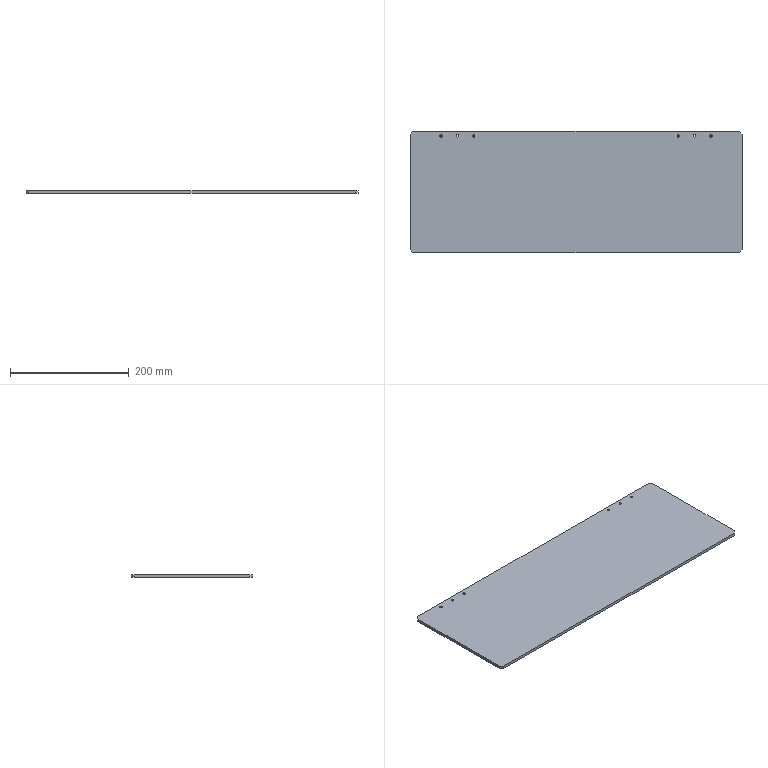Part | SolidWorks | features Extrusion 1 | 1 solid | 22 faces | box 560 x 205 x 5 mm | volume 573373 mm3 | cylinder 12 | plane 10 | commonest cylinder face diameters 4 x12
STEP:
#1=CARTESIAN_POINT('',(505.5,-8.,5.));
#2=VERTEX_POINT('',#1);
#3=CARTESIAN_POINT('',(509.5,-8.,5.));
#4=VERTEX_POINT('',#3);
#5=CARTESIAN_POINT('',(507.5,-8.,5.));
#6=DIRECTION('',(0.,0.,1.));
#7=DIRECTION('',(-1.,0.,0.));
#8=AXIS2_PLACEMENT_3D('',#5,#6,#7);
#9=CIRCLE('',#8,2.);
#10=EDGE_CURVE('',#2,#4,#9,.T.);
#11=ORIENTED_EDGE('',*,*,#10,.T.);
#12=CARTESIAN_POINT('',(509.5,-8.,0.));
#13=VERTEX_POINT('',#12);
#14=CARTESIAN_POINT('',(509.5,-8.,5.));
#15=DIRECTION('',(0.,0.,-1.));
#16=VECTOR('',#15,1000.);
#17=LINE('',#14,#16);
#18=EDGE_CURVE('',#4,#13,#17,.T.);
#19=ORIENTED_EDGE('',*,*,#18,.T.);
#20=CARTESIAN_POINT('',(505.5,-8.,0.));
#21=VERTEX_POINT('',#20);
#22=CARTESIAN_POINT('',(507.5,-8.,0.));
#23=DIRECTION('',(0.,0.,1.));
#24=DIRECTION('',(-1.,0.,0.));
#25=AXIS2_PLACEMENT_3D('',#22,#23,#24);
#26=CIRCLE('',#25,2.);
#27=EDGE_CURVE('',#21,#13,#26,.T.);
#28=ORIENTED_EDGE('',*,*,#27,.F.);
#29=CARTESIAN_POINT('',(505.5,-8.,5.));
#30=DIRECTION('',(0.,0.,-1.));
#31=VECTOR('',#30,1000.);
#32=LINE('',#29,#31);
#33=EDGE_CURVE('',#2,#21,#32,.T.);
#34=ORIENTED_EDGE('',*,*,#33,.F.);
#35=EDGE_LOOP('',(#11,#19,#28,#34));
#36=FACE_OUTER_BOUND('',#35,.T.);
#37=CARTESIAN_POINT('',(507.5,-8.,5.));
#38=DIRECTION('',(0.,0.,-1.));
#39=DIRECTION('',(-1.,0.,0.));
#40=AXIS2_PLACEMENT_3D('',#37,#38,#39);
#41=CYLINDRICAL_SURFACE('',#40,2.);
#42=ADVANCED_FACE('',(#36),#41,.F.);
#43=CARTESIAN_POINT('',(478.,-8.,5.));
#44=VERTEX_POINT('',#43);
#45=CARTESIAN_POINT('',(482.,-8.,5.));
#46=VERTEX_POINT('',#45);
#47=CARTESIAN_POINT('',(480.,-8.,5.));
#48=DIRECTION('',(0.,0.,1.));
#49=DIRECTION('',(-1.,0.,0.));
#50=AXIS2_PLACEMENT_3D('',#47,#48,#49);
#51=CIRCLE('',#50,2.);
#52=EDGE_CURVE('',#44,#46,#51,.T.);
#53=ORIENTED_EDGE('',*,*,#52,.T.);
#54=CARTESIAN_POINT('',(482.,-8.,0.));
#55=VERTEX_POINT('',#54);
#56=CARTESIAN_POINT('',(482.,-8.,5.));
#57=DIRECTION('',(0.,0.,-1.));
#58=VECTOR('',#57,1000.);
#59=LINE('',#56,#58);
#60=EDGE_CURVE('',#46,#55,#59,.T.);
#61=ORIENTED_EDGE('',*,*,#60,.T.);
#62=CARTESIAN_POINT('',(478.,-8.,0.));
#63=VERTEX_POINT('',#62);
#64=CARTESIAN_POINT('',(480.,-8.,0.));
#65=DIRECTION('',(0.,0.,1.));
#66=DIRECTION('',(-1.,0.,0.));
#67=AXIS2_PLACEMENT_3D('',#64,#65,#66);
#68=CIRCLE('',#67,2.);
#69=EDGE_CURVE('',#63,#55,#68,.T.);
#70=ORIENTED_EDGE('',*,*,#69,.F.);
#71=CARTESIAN_POINT('',(478.,-8.,5.));
#72=DIRECTION('',(0.,0.,-1.));
#73=VECTOR('',#72,1000.);
#74=LINE('',#71,#73);
#75=EDGE_CURVE('',#44,#63,#74,.T.);
#76=ORIENTED_EDGE('',*,*,#75,.F.);
#77=EDGE_LOOP('',(#53,#61,#70,#76));
#78=FACE_OUTER_BOUND('',#77,.T.);
#79=CARTESIAN_POINT('',(480.,-8.,5.));
#80=DIRECTION('',(0.,0.,-1.));
#81=DIRECTION('',(-1.,0.,0.));
#82=AXIS2_PLACEMENT_3D('',#79,#80,#81);
#83=CYLINDRICAL_SURFACE('',#82,2.);
#84=ADVANCED_FACE('',(#78),#83,.F.);
#85=CARTESIAN_POINT('',(450.5,-8.,5.));
#86=VERTEX_POINT('',#85);
#87=CARTESIAN_POINT('',(454.5,-8.,5.));
#88=VERTEX_POINT('',#87);
#89=CARTESIAN_POINT('',(452.5,-8.,5.));
#90=DIRECTION('',(0.,0.,1.));
#91=DIRECTION('',(-1.,0.,0.));
#92=AXIS2_PLACEMENT_3D('',#89,#90,#91);
#93=CIRCLE('',#92,2.);
#94=EDGE_CURVE('',#86,#88,#93,.T.);
#95=ORIENTED_EDGE('',*,*,#94,.T.);
#96=CARTESIAN_POINT('',(454.5,-8.,0.));
#97=VERTEX_POINT('',#96);
#98=CARTESIAN_POINT('',(454.5,-8.,5.));
#99=DIRECTION('',(0.,0.,-1.));
#100=VECTOR('',#99,1000.);
#101=LINE('',#98,#100);
#102=EDGE_CURVE('',#88,#97,#101,.T.);
#103=ORIENTED_EDGE('',*,*,#102,.T.);
#104=CARTESIAN_POINT('',(450.5,-8.,0.));
#105=VERTEX_POINT('',#104);
#106=CARTESIAN_POINT('',(452.5,-8.,0.));
#107=DIRECTION('',(0.,0.,1.));
#108=DIRECTION('',(-1.,0.,0.));
#109=AXIS2_PLACEMENT_3D('',#106,#107,#108);
#110=CIRCLE('',#109,2.);
#111=EDGE_CURVE('',#105,#97,#110,.T.);
#112=ORIENTED_EDGE('',*,*,#111,.F.);
#113=CARTESIAN_POINT('',(450.5,-8.,5.));
#114=DIRECTION('',(0.,0.,-1.));
#115=VECTOR('',#114,1000.);
#116=LINE('',#113,#115);
#117=EDGE_CURVE('',#86,#105,#116,.T.);
#118=ORIENTED_EDGE('',*,*,#117,.F.);
#119=EDGE_LOOP('',(#95,#103,#112,#118));
#120=FACE_OUTER_BOUND('',#119,.T.);
#121=CARTESIAN_POINT('',(452.5,-8.,5.));
#122=DIRECTION('',(0.,0.,-1.));
#123=DIRECTION('',(-1.,0.,0.));
#124=AXIS2_PLACEMENT_3D('',#121,#122,#123);
#125=CYLINDRICAL_SURFACE('',#124,2.);
#126=ADVANCED_FACE('',(#120),#125,.F.);
#127=CARTESIAN_POINT('',(105.5,-8.,5.));
#128=VERTEX_POINT('',#127);
#129=CARTESIAN_POINT('',(109.5,-8.,5.));
#130=VERTEX_POINT('',#129);
#131=CARTESIAN_POINT('',(107.5,-8.,5.));
#132=DIRECTION('',(0.,0.,1.));
#133=DIRECTION('',(1.,0.,0.));
#134=AXIS2_PLACEMENT_3D('',#131,#132,#133);
#135=CIRCLE('',#134,2.);
#136=EDGE_CURVE('',#128,#130,#135,.T.);
#137=ORIENTED_EDGE('',*,*,#136,.T.);
#138=CARTESIAN_POINT('',(109.5,-8.,0.));
#139=VERTEX_POINT('',#138);
#140=CARTESIAN_POINT('',(109.5,-8.,5.));
#141=DIRECTION('',(0.,0.,-1.));
#142=VECTOR('',#141,1000.);
#143=LINE('',#140,#142);
#144=EDGE_CURVE('',#130,#139,#143,.T.);
#145=ORIENTED_EDGE('',*,*,#144,.T.);
#146=CARTESIAN_POINT('',(105.5,-8.,0.));
#147=VERTEX_POINT('',#146);
#148=CARTESIAN_POINT('',(107.5,-8.,0.));
#149=DIRECTION('',(0.,0.,1.));
#150=DIRECTION('',(1.,0.,0.));
#151=AXIS2_PLACEMENT_3D('',#148,#149,#150);
#152=CIRCLE('',#151,2.);
#153=EDGE_CURVE('',#147,#139,#152,.T.);
#154=ORIENTED_EDGE('',*,*,#153,.F.);
#155=CARTESIAN_POINT('',(105.5,-8.,5.));
#156=DIRECTION('',(0.,0.,-1.));
#157=VECTOR('',#156,1000.);
#158=LINE('',#155,#157);
#159=EDGE_CURVE('',#128,#147,#158,.T.);
#160=ORIENTED_EDGE('',*,*,#159,.F.);
#161=EDGE_LOOP('',(#137,#145,#154,#160));
#162=FACE_OUTER_BOUND('',#161,.T.);
#163=CARTESIAN_POINT('',(107.5,-8.,5.));
#164=DIRECTION('',(0.,0.,-1.));
#165=DIRECTION('',(-1.,0.,0.));
#166=AXIS2_PLACEMENT_3D('',#163,#164,#165);
#167=CYLINDRICAL_SURFACE('',#166,2.);
#168=ADVANCED_FACE('',(#162),#167,.F.);
#169=CARTESIAN_POINT('',(78.,-8.,5.));
#170=VERTEX_POINT('',#169);
#171=CARTESIAN_POINT('',(82.,-8.,5.));
#172=VERTEX_POINT('',#171);
#173=CARTESIAN_POINT('',(80.,-8.,5.));
#174=DIRECTION('',(0.,0.,1.));
#175=DIRECTION('',(1.,0.,0.));
#176=AXIS2_PLACEMENT_3D('',#173,#174,#175);
#177=CIRCLE('',#176,2.);
#178=EDGE_CURVE('',#170,#172,#177,.T.);
#179=ORIENTED_EDGE('',*,*,#178,.T.);
#180=CARTESIAN_POINT('',(82.,-8.,0.));
#181=VERTEX_POINT('',#180);
#182=CARTESIAN_POINT('',(82.,-8.,5.));
#183=DIRECTION('',(0.,0.,-1.));
#184=VECTOR('',#183,1000.);
#185=LINE('',#182,#184);
#186=EDGE_CURVE('',#172,#181,#185,.T.);
#187=ORIENTED_EDGE('',*,*,#186,.T.);
#188=CARTESIAN_POINT('',(78.,-8.,0.));
#189=VERTEX_POINT('',#188);
#190=CARTESIAN_POINT('',(80.,-8.,0.));
#191=DIRECTION('',(0.,0.,1.));
#192=DIRECTION('',(1.,0.,0.));
#193=AXIS2_PLACEMENT_3D('',#190,#191,#192);
#194=CIRCLE('',#193,2.);
#195=EDGE_CURVE('',#189,#181,#194,.T.);
#196=ORIENTED_EDGE('',*,*,#195,.F.);
#197=CARTESIAN_POINT('',(78.,-8.,5.));
#198=DIRECTION('',(0.,0.,-1.));
#199=VECTOR('',#198,1000.);
#200=LINE('',#197,#199);
#201=EDGE_CURVE('',#170,#189,#200,.T.);
#202=ORIENTED_EDGE('',*,*,#201,.F.);
#203=EDGE_LOOP('',(#179,#187,#196,#202));
#204=FACE_OUTER_BOUND('',#203,.T.);
#205=CARTESIAN_POINT('',(80.,-8.,5.));
#206=DIRECTION('',(0.,0.,-1.));
#207=DIRECTION('',(-1.,0.,0.));
#208=AXIS2_PLACEMENT_3D('',#205,#206,#207);
#209=CYLINDRICAL_SURFACE('',#208,2.);
#210=ADVANCED_FACE('',(#204),#209,.F.);
#211=CARTESIAN_POINT('',(50.5,-8.,5.));
#212=VERTEX_POINT('',#211);
#213=CARTESIAN_POINT('',(54.5,-8.,5.));
#214=VERTEX_POINT('',#213);
#215=CARTESIAN_POINT('',(52.5,-8.,5.));
#216=DIRECTION('',(0.,0.,1.));
#217=DIRECTION('',(1.,0.,0.));
#218=AXIS2_PLACEMENT_3D('',#215,#216,#217);
#219=CIRCLE('',#218,2.);
#220=EDGE_CURVE('',#212,#214,#219,.T.);
#221=ORIENTED_EDGE('',*,*,#220,.T.);
#222=CARTESIAN_POINT('',(54.5,-8.,0.));
#223=VERTEX_POINT('',#222);
#224=CARTESIAN_POINT('',(54.5,-8.,5.));
#225=DIRECTION('',(0.,0.,-1.));
#226=VECTOR('',#225,1000.);
#227=LINE('',#224,#226);
#228=EDGE_CURVE('',#214,#223,#227,.T.);
#229=ORIENTED_EDGE('',*,*,#228,.T.);
#230=CARTESIAN_POINT('',(50.5,-8.,0.));
#231=VERTEX_POINT('',#230);
#232=CARTESIAN_POINT('',(52.5,-8.,0.));
#233=DIRECTION('',(0.,0.,1.));
#234=DIRECTION('',(1.,0.,0.));
#235=AXIS2_PLACEMENT_3D('',#232,#233,#234);
#236=CIRCLE('',#235,2.);
#237=EDGE_CURVE('',#231,#223,#236,.T.);
#238=ORIENTED_EDGE('',*,*,#237,.F.);
#239=CARTESIAN_POINT('',(50.5,-8.,5.));
#240=DIRECTION('',(0.,0.,-1.));
#241=VECTOR('',#240,1000.);
#242=LINE('',#239,#241);
#243=EDGE_CURVE('',#212,#231,#242,.T.);
#244=ORIENTED_EDGE('',*,*,#243,.F.);
#245=EDGE_LOOP('',(#221,#229,#238,#244));
#246=FACE_OUTER_BOUND('',#245,.T.);
#247=CARTESIAN_POINT('',(52.5,-8.,5.));
#248=DIRECTION('',(0.,0.,-1.));
#249=DIRECTION('',(-1.,0.,0.));
#250=AXIS2_PLACEMENT_3D('',#247,#248,#249);
#251=CYLINDRICAL_SURFACE('',#250,2.);
#252=ADVANCED_FACE('',(#246),#251,.F.);
#253=CARTESIAN_POINT('',(555.,0.,5.));
#254=VERTEX_POINT('',#253);
#255=CARTESIAN_POINT('',(5.,0.,5.));
#256=VERTEX_POINT('',#255);
#257=CARTESIAN_POINT('',(5.,0.,5.));
#258=DIRECTION('',(-1.,0.,0.));
#259=VECTOR('',#258,1000.);
#260=LINE('',#257,#259);
#261=EDGE_CURVE('',#254,#256,#260,.T.);
#262=ORIENTED_EDGE('',*,*,#261,.T.);
#263=CARTESIAN_POINT('',(0.,-5.,5.));
#264=VERTEX_POINT('',#263);
#265=CARTESIAN_POINT('',(0.,-5.,5.));
#266=DIRECTION('',(-0.7071,-0.7071,0.));
#267=VECTOR('',#266,1000.);
#268=LINE('',#265,#267);
#269=EDGE_CURVE('',#256,#264,#268,.T.);
#270=ORIENTED_EDGE('',*,*,#269,.T.);
#271=CARTESIAN_POINT('',(0.,-200.,5.));
#272=VERTEX_POINT('',#271);
#273=CARTESIAN_POINT('',(0.,-5.,5.));
#274=DIRECTION('',(0.,-1.,0.));
#275=VECTOR('',#274,1000.);
#276=LINE('',#273,#275);
#277=EDGE_CURVE('',#264,#272,#276,.T.);
#278=ORIENTED_EDGE('',*,*,#277,.T.);
#279=CARTESIAN_POINT('',(5.,-205.,5.));
#280=VERTEX_POINT('',#279);
#281=CARTESIAN_POINT('',(0.,-200.,5.));
#282=DIRECTION('',(0.7071,-0.7071,0.));
#283=VECTOR('',#282,1000.);
#284=LINE('',#281,#283);
#285=EDGE_CURVE('',#272,#280,#284,.T.);
#286=ORIENTED_EDGE('',*,*,#285,.T.);
#287=CARTESIAN_POINT('',(555.,-205.,5.));
#288=VERTEX_POINT('',#287);
#289=CARTESIAN_POINT('',(5.,-205.,5.));
#290=DIRECTION('',(1.,0.,0.));
#291=VECTOR('',#290,1000.);
#292=LINE('',#289,#291);
#293=EDGE_CURVE('',#280,#288,#292,.T.);
#294=ORIENTED_EDGE('',*,*,#293,.T.);
#295=CARTESIAN_POINT('',(560.,-200.,5.));
#296=VERTEX_POINT('',#295);
#297=CARTESIAN_POINT('',(560.,-200.,5.));
#298=DIRECTION('',(0.7071,0.7071,0.));
#299=VECTOR('',#298,1000.);
#300=LINE('',#297,#299);
#301=EDGE_CURVE('',#288,#296,#300,.T.);
#302=ORIENTED_EDGE('',*,*,#301,.T.);
#303=CARTESIAN_POINT('',(560.,-5.,5.));
#304=VERTEX_POINT('',#303);
#305=CARTESIAN_POINT('',(560.,-5.,5.));
#306=DIRECTION('',(0.,1.,0.));
#307=VECTOR('',#306,1000.);
#308=LINE('',#305,#307);
#309=EDGE_CURVE('',#296,#304,#308,.T.);
#310=ORIENTED_EDGE('',*,*,#309,.T.);
#311=CARTESIAN_POINT('',(555.,0.,5.));
#312=DIRECTION('',(-0.7071,0.7071,0.));
#313=VECTOR('',#312,1000.);
#314=LINE('',#311,#313);
#315=EDGE_CURVE('',#304,#254,#314,.T.);
#316=ORIENTED_EDGE('',*,*,#315,.T.);
#317=EDGE_LOOP('',(#262,#270,#278,#286,#294,#302,#310,#316));
#318=FACE_OUTER_BOUND('',#317,.T.);
#319=ORIENTED_EDGE('',*,*,#220,.F.);
#320=CARTESIAN_POINT('',(52.5,-8.,5.));
#321=DIRECTION('',(0.,0.,1.));
#322=DIRECTION('',(1.,0.,0.));
#323=AXIS2_PLACEMENT_3D('',#320,#321,#322);
#324=CIRCLE('',#323,2.);
#325=EDGE_CURVE('',#214,#212,#324,.T.);
#326=ORIENTED_EDGE('',*,*,#325,.F.);
#327=EDGE_LOOP('',(#319,#326));
#328=FACE_BOUND('',#327,.T.);
#329=ORIENTED_EDGE('',*,*,#178,.F.);
#330=CARTESIAN_POINT('',(80.,-8.,5.));
#331=DIRECTION('',(0.,0.,1.));
#332=DIRECTION('',(1.,0.,0.));
#333=AXIS2_PLACEMENT_3D('',#330,#331,#332);
#334=CIRCLE('',#333,2.);
#335=EDGE_CURVE('',#172,#170,#334,.T.);
#336=ORIENTED_EDGE('',*,*,#335,.F.);
#337=EDGE_LOOP('',(#329,#336));
#338=FACE_BOUND('',#337,.T.);
#339=ORIENTED_EDGE('',*,*,#136,.F.);
#340=CARTESIAN_POINT('',(107.5,-8.,5.));
#341=DIRECTION('',(0.,0.,1.));
#342=DIRECTION('',(1.,0.,0.));
#343=AXIS2_PLACEMENT_3D('',#340,#341,#342);
#344=CIRCLE('',#343,2.);
#345=EDGE_CURVE('',#130,#128,#344,.T.);
#346=ORIENTED_EDGE('',*,*,#345,.F.);
#347=EDGE_LOOP('',(#339,#346));
#348=FACE_BOUND('',#347,.T.);
#349=ORIENTED_EDGE('',*,*,#94,.F.);
#350=CARTESIAN_POINT('',(452.5,-8.,5.));
#351=DIRECTION('',(0.,0.,1.));
#352=DIRECTION('',(-1.,0.,0.));
#353=AXIS2_PLACEMENT_3D('',#350,#351,#352);
#354=CIRCLE('',#353,2.);
#355=EDGE_CURVE('',#88,#86,#354,.T.);
#356=ORIENTED_EDGE('',*,*,#355,.F.);
#357=EDGE_LOOP('',(#349,#356));
#358=FACE_BOUND('',#357,.T.);
#359=ORIENTED_EDGE('',*,*,#52,.F.);
#360=CARTESIAN_POINT('',(480.,-8.,5.));
#361=DIRECTION('',(0.,0.,1.));
#362=DIRECTION('',(-1.,0.,0.));
#363=AXIS2_PLACEMENT_3D('',#360,#361,#362);
#364=CIRCLE('',#363,2.);
#365=EDGE_CURVE('',#46,#44,#364,.T.);
#366=ORIENTED_EDGE('',*,*,#365,.F.);
#367=EDGE_LOOP('',(#359,#366));
#368=FACE_BOUND('',#367,.T.);
#369=ORIENTED_EDGE('',*,*,#10,.F.);
#370=CARTESIAN_POINT('',(507.5,-8.,5.));
#371=DIRECTION('',(0.,0.,1.));
#372=DIRECTION('',(-1.,0.,0.));
#373=AXIS2_PLACEMENT_3D('',#370,#371,#372);
#374=CIRCLE('',#373,2.);
#375=EDGE_CURVE('',#4,#2,#374,.T.);
#376=ORIENTED_EDGE('',*,*,#375,.F.);
#377=EDGE_LOOP('',(#369,#376));
#378=FACE_BOUND('',#377,.T.);
#379=CARTESIAN_POINT('',(0.,0.,5.));
#380=DIRECTION('',(0.,0.,-1.));
#381=DIRECTION('',(-1.,0.,0.));
#382=AXIS2_PLACEMENT_3D('',#379,#380,#381);
#383=PLANE('',#382);
#384=ADVANCED_FACE('',(#318,#328,#338,#348,#358,#368,#378),#383,.F.);
#385=ORIENTED_EDGE('',*,*,#69,.T.);
#386=CARTESIAN_POINT('',(480.,-8.,0.));
#387=DIRECTION('',(0.,0.,1.));
#388=DIRECTION('',(-1.,0.,0.));
#389=AXIS2_PLACEMENT_3D('',#386,#387,#388);
#390=CIRCLE('',#389,2.);
#391=EDGE_CURVE('',#55,#63,#390,.T.);
#392=ORIENTED_EDGE('',*,*,#391,.T.);
#393=EDGE_LOOP('',(#385,#392));
#394=FACE_BOUND('',#393,.T.);
#395=ORIENTED_EDGE('',*,*,#153,.T.);
#396=CARTESIAN_POINT('',(107.5,-8.,0.));
#397=DIRECTION('',(0.,0.,1.));
#398=DIRECTION('',(1.,0.,0.));
#399=AXIS2_PLACEMENT_3D('',#396,#397,#398);
#400=CIRCLE('',#399,2.);
#401=EDGE_CURVE('',#139,#147,#400,.T.);
#402=ORIENTED_EDGE('',*,*,#401,.T.);
#403=EDGE_LOOP('',(#395,#402));
#404=FACE_BOUND('',#403,.T.);
#405=ORIENTED_EDGE('',*,*,#237,.T.);
#406=CARTESIAN_POINT('',(52.5,-8.,0.));
#407=DIRECTION('',(0.,0.,1.));
#408=DIRECTION('',(1.,0.,0.));
#409=AXIS2_PLACEMENT_3D('',#406,#407,#408);
#410=CIRCLE('',#409,2.);
#411=EDGE_CURVE('',#223,#231,#410,.T.);
#412=ORIENTED_EDGE('',*,*,#411,.T.);
#413=EDGE_LOOP('',(#405,#412));
#414=FACE_BOUND('',#413,.T.);
#415=CARTESIAN_POINT('',(555.,0.,0.));
#416=VERTEX_POINT('',#415);
#417=CARTESIAN_POINT('',(5.,0.,0.));
#418=VERTEX_POINT('',#417);
#419=CARTESIAN_POINT('',(5.,0.,0.));
#420=DIRECTION('',(-1.,0.,0.));
#421=VECTOR('',#420,1000.);
#422=LINE('',#419,#421);
#423=EDGE_CURVE('',#416,#418,#422,.T.);
#424=ORIENTED_EDGE('',*,*,#423,.F.);
#425=CARTESIAN_POINT('',(560.,-5.,0.));
#426=VERTEX_POINT('',#425);
#427=CARTESIAN_POINT('',(555.,0.,0.));
#428=DIRECTION('',(-0.7071,0.7071,0.));
#429=VECTOR('',#428,1000.);
#430=LINE('',#427,#429);
#431=EDGE_CURVE('',#426,#416,#430,.T.);
#432=ORIENTED_EDGE('',*,*,#431,.F.);
#433=CARTESIAN_POINT('',(560.,-200.,0.));
#434=VERTEX_POINT('',#433);
#435=CARTESIAN_POINT('',(560.,-5.,0.));
#436=DIRECTION('',(0.,1.,0.));
#437=VECTOR('',#436,1000.);
#438=LINE('',#435,#437);
#439=EDGE_CURVE('',#434,#426,#438,.T.);
#440=ORIENTED_EDGE('',*,*,#439,.F.);
#441=CARTESIAN_POINT('',(555.,-205.,0.));
#442=VERTEX_POINT('',#441);
#443=CARTESIAN_POINT('',(560.,-200.,0.));
#444=DIRECTION('',(0.7071,0.7071,0.));
#445=VECTOR('',#444,1000.);
#446=LINE('',#443,#445);
#447=EDGE_CURVE('',#442,#434,#446,.T.);
#448=ORIENTED_EDGE('',*,*,#447,.F.);
#449=CARTESIAN_POINT('',(5.,-205.,0.));
#450=VERTEX_POINT('',#449);
#451=CARTESIAN_POINT('',(5.,-205.,0.));
#452=DIRECTION('',(1.,0.,0.));
#453=VECTOR('',#452,1000.);
#454=LINE('',#451,#453);
#455=EDGE_CURVE('',#450,#442,#454,.T.);
#456=ORIENTED_EDGE('',*,*,#455,.F.);
#457=CARTESIAN_POINT('',(0.,-200.,0.));
#458=VERTEX_POINT('',#457);
#459=CARTESIAN_POINT('',(0.,-200.,0.));
#460=DIRECTION('',(0.7071,-0.7071,0.));
#461=VECTOR('',#460,1000.);
#462=LINE('',#459,#461);
#463=EDGE_CURVE('',#458,#450,#462,.T.);
#464=ORIENTED_EDGE('',*,*,#463,.F.);
#465=CARTESIAN_POINT('',(0.,-5.,0.));
#466=VERTEX_POINT('',#465);
#467=CARTESIAN_POINT('',(0.,-5.,0.));
#468=DIRECTION('',(0.,-1.,0.));
#469=VECTOR('',#468,1000.);
#470=LINE('',#467,#469);
#471=EDGE_CURVE('',#466,#458,#470,.T.);
#472=ORIENTED_EDGE('',*,*,#471,.F.);
#473=CARTESIAN_POINT('',(0.,-5.,0.));
#474=DIRECTION('',(-0.7071,-0.7071,0.));
#475=VECTOR('',#474,1000.);
#476=LINE('',#473,#475);
#477=EDGE_CURVE('',#418,#466,#476,.T.);
#478=ORIENTED_EDGE('',*,*,#477,.F.);
#479=EDGE_LOOP('',(#424,#432,#440,#448,#456,#464,#472,#478));
#480=FACE_OUTER_BOUND('',#479,.T.);
#481=ORIENTED_EDGE('',*,*,#195,.T.);
#482=CARTESIAN_POINT('',(80.,-8.,0.));
#483=DIRECTION('',(0.,0.,1.));
#484=DIRECTION('',(1.,0.,0.));
#485=AXIS2_PLACEMENT_3D('',#482,#483,#484);
#486=CIRCLE('',#485,2.);
#487=EDGE_CURVE('',#181,#189,#486,.T.);
#488=ORIENTED_EDGE('',*,*,#487,.T.);
#489=EDGE_LOOP('',(#481,#488));
#490=FACE_BOUND('',#489,.T.);
#491=ORIENTED_EDGE('',*,*,#111,.T.);
#492=CARTESIAN_POINT('',(452.5,-8.,0.));
#493=DIRECTION('',(0.,0.,1.));
#494=DIRECTION('',(-1.,0.,0.));
#495=AXIS2_PLACEMENT_3D('',#492,#493,#494);
#496=CIRCLE('',#495,2.);
#497=EDGE_CURVE('',#97,#105,#496,.T.);
#498=ORIENTED_EDGE('',*,*,#497,.T.);
#499=EDGE_LOOP('',(#491,#498));
#500=FACE_BOUND('',#499,.T.);
#501=ORIENTED_EDGE('',*,*,#27,.T.);
#502=CARTESIAN_POINT('',(507.5,-8.,0.));
#503=DIRECTION('',(0.,0.,1.));
#504=DIRECTION('',(-1.,0.,0.));
#505=AXIS2_PLACEMENT_3D('',#502,#503,#504);
#506=CIRCLE('',#505,2.);
#507=EDGE_CURVE('',#13,#21,#506,.T.);
#508=ORIENTED_EDGE('',*,*,#507,.T.);
#509=EDGE_LOOP('',(#501,#508));
#510=FACE_BOUND('',#509,.T.);
#511=CARTESIAN_POINT('',(0.,0.,0.));
#512=DIRECTION('',(0.,0.,-1.));
#513=DIRECTION('',(-1.,0.,0.));
#514=AXIS2_PLACEMENT_3D('',#511,#512,#513);
#515=PLANE('',#514);
#516=ADVANCED_FACE('',(#394,#404,#414,#480,#490,#500,#510),#515,.T.);
#517=ORIENTED_EDGE('',*,*,#423,.T.);
#518=CARTESIAN_POINT('',(5.,0.,5.));
#519=DIRECTION('',(0.,0.,-1.));
#520=VECTOR('',#519,1000.);
#521=LINE('',#518,#520);
#522=EDGE_CURVE('',#256,#418,#521,.T.);
#523=ORIENTED_EDGE('',*,*,#522,.F.);
#524=ORIENTED_EDGE('',*,*,#261,.F.);
#525=CARTESIAN_POINT('',(555.,0.,5.));
#526=DIRECTION('',(0.,0.,-1.));
#527=VECTOR('',#526,1000.);
#528=LINE('',#525,#527);
#529=EDGE_CURVE('',#254,#416,#528,.T.);
#530=ORIENTED_EDGE('',*,*,#529,.T.);
#531=EDGE_LOOP('',(#517,#523,#524,#530));
#532=FACE_OUTER_BOUND('',#531,.T.);
#533=CARTESIAN_POINT('',(5.,0.,5.));
#534=DIRECTION('',(0.,-1.,0.));
#535=DIRECTION('',(1.,0.,0.));
#536=AXIS2_PLACEMENT_3D('',#533,#534,#535);
#537=PLANE('',#536);
#538=ADVANCED_FACE('',(#532),#537,.F.);
#539=ORIENTED_EDGE('',*,*,#477,.T.);
#540=CARTESIAN_POINT('',(0.,-5.,5.));
#541=DIRECTION('',(0.,0.,-1.));
#542=VECTOR('',#541,1000.);
#543=LINE('',#540,#542);
#544=EDGE_CURVE('',#264,#466,#543,.T.);
#545=ORIENTED_EDGE('',*,*,#544,.F.);
#546=ORIENTED_EDGE('',*,*,#269,.F.);
#547=ORIENTED_EDGE('',*,*,#522,.T.);
#548=EDGE_LOOP('',(#539,#545,#546,#547));
#549=FACE_OUTER_BOUND('',#548,.T.);
#550=CARTESIAN_POINT('',(0.,-5.,5.));
#551=DIRECTION('',(0.7071,-0.7071,0.));
#552=DIRECTION('',(0.7071,0.7071,0.));
#553=AXIS2_PLACEMENT_3D('',#550,#551,#552);
#554=PLANE('',#553);
#555=ADVANCED_FACE('',(#549),#554,.F.);
#556=ORIENTED_EDGE('',*,*,#471,.T.);
#557=CARTESIAN_POINT('',(0.,-200.,5.));
#558=DIRECTION('',(0.,0.,-1.));
#559=VECTOR('',#558,1000.);
#560=LINE('',#557,#559);
#561=EDGE_CURVE('',#272,#458,#560,.T.);
#562=ORIENTED_EDGE('',*,*,#561,.F.);
#563=ORIENTED_EDGE('',*,*,#277,.F.);
#564=ORIENTED_EDGE('',*,*,#544,.T.);
#565=EDGE_LOOP('',(#556,#562,#563,#564));
#566=FACE_OUTER_BOUND('',#565,.T.);
#567=CARTESIAN_POINT('',(0.,-5.,5.));
#568=DIRECTION('',(1.,0.,0.));
#569=DIRECTION('',(0.,1.,0.));
#570=AXIS2_PLACEMENT_3D('',#567,#568,#569);
#571=PLANE('',#570);
#572=ADVANCED_FACE('',(#566),#571,.F.);
#573=ORIENTED_EDGE('',*,*,#463,.T.);
#574=CARTESIAN_POINT('',(5.,-205.,5.));
#575=DIRECTION('',(0.,0.,-1.));
#576=VECTOR('',#575,1000.);
#577=LINE('',#574,#576);
#578=EDGE_CURVE('',#280,#450,#577,.T.);
#579=ORIENTED_EDGE('',*,*,#578,.F.);
#580=ORIENTED_EDGE('',*,*,#285,.F.);
#581=ORIENTED_EDGE('',*,*,#561,.T.);
#582=EDGE_LOOP('',(#573,#579,#580,#581));
#583=FACE_OUTER_BOUND('',#582,.T.);
#584=CARTESIAN_POINT('',(0.,-200.,5.));
#585=DIRECTION('',(0.7071,0.7071,0.));
#586=DIRECTION('',(-0.7071,0.7071,0.));
#587=AXIS2_PLACEMENT_3D('',#584,#585,#586);
#588=PLANE('',#587);
#589=ADVANCED_FACE('',(#583),#588,.F.);
#590=ORIENTED_EDGE('',*,*,#455,.T.);
#591=CARTESIAN_POINT('',(555.,-205.,5.));
#592=DIRECTION('',(0.,0.,-1.));
#593=VECTOR('',#592,1000.);
#594=LINE('',#591,#593);
#595=EDGE_CURVE('',#288,#442,#594,.T.);
#596=ORIENTED_EDGE('',*,*,#595,.F.);
#597=ORIENTED_EDGE('',*,*,#293,.F.);
#598=ORIENTED_EDGE('',*,*,#578,.T.);
#599=EDGE_LOOP('',(#590,#596,#597,#598));
#600=FACE_OUTER_BOUND('',#599,.T.);
#601=CARTESIAN_POINT('',(5.,-205.,5.));
#602=DIRECTION('',(0.,1.,0.));
#603=DIRECTION('',(0.,0.,1.));
#604=AXIS2_PLACEMENT_3D('',#601,#602,#603);
#605=PLANE('',#604);
#606=ADVANCED_FACE('',(#600),#605,.F.);
#607=ORIENTED_EDGE('',*,*,#447,.T.);
#608=CARTESIAN_POINT('',(560.,-200.,5.));
#609=DIRECTION('',(0.,0.,-1.));
#610=VECTOR('',#609,1000.);
#611=LINE('',#608,#610);
#612=EDGE_CURVE('',#296,#434,#611,.T.);
#613=ORIENTED_EDGE('',*,*,#612,.F.);
#614=ORIENTED_EDGE('',*,*,#301,.F.);
#615=ORIENTED_EDGE('',*,*,#595,.T.);
#616=EDGE_LOOP('',(#607,#613,#614,#615));
#617=FACE_OUTER_BOUND('',#616,.T.);
#618=CARTESIAN_POINT('',(560.,-200.,5.));
#619=DIRECTION('',(-0.7071,0.7071,0.));
#620=DIRECTION('',(-0.7071,-0.7071,0.));
#621=AXIS2_PLACEMENT_3D('',#618,#619,#620);
#622=PLANE('',#621);
#623=ADVANCED_FACE('',(#617),#622,.F.);
#624=ORIENTED_EDGE('',*,*,#439,.T.);
#625=CARTESIAN_POINT('',(560.,-5.,5.));
#626=DIRECTION('',(0.,0.,-1.));
#627=VECTOR('',#626,1000.);
#628=LINE('',#625,#627);
#629=EDGE_CURVE('',#304,#426,#628,.T.);
#630=ORIENTED_EDGE('',*,*,#629,.F.);
#631=ORIENTED_EDGE('',*,*,#309,.F.);
#632=ORIENTED_EDGE('',*,*,#612,.T.);
#633=EDGE_LOOP('',(#624,#630,#631,#632));
#634=FACE_OUTER_BOUND('',#633,.T.);
#635=CARTESIAN_POINT('',(560.,-5.,5.));
#636=DIRECTION('',(-1.,0.,0.));
#637=DIRECTION('',(0.,0.,1.));
#638=AXIS2_PLACEMENT_3D('',#635,#636,#637);
#639=PLANE('',#638);
#640=ADVANCED_FACE('',(#634),#639,.F.);
#641=ORIENTED_EDGE('',*,*,#431,.T.);
#642=ORIENTED_EDGE('',*,*,#529,.F.);
#643=ORIENTED_EDGE('',*,*,#315,.F.);
#644=ORIENTED_EDGE('',*,*,#629,.T.);
#645=EDGE_LOOP('',(#641,#642,#643,#644));
#646=FACE_OUTER_BOUND('',#645,.T.);
#647=CARTESIAN_POINT('',(555.,0.,5.));
#648=DIRECTION('',(-0.7071,-0.7071,0.));
#649=DIRECTION('',(0.7071,-0.7071,0.));
#650=AXIS2_PLACEMENT_3D('',#647,#648,#649);
#651=PLANE('',#650);
#652=ADVANCED_FACE('',(#646),#651,.F.);
#653=ORIENTED_EDGE('',*,*,#228,.F.);
#654=ORIENTED_EDGE('',*,*,#325,.T.);
#655=ORIENTED_EDGE('',*,*,#243,.T.);
#656=ORIENTED_EDGE('',*,*,#411,.F.);
#657=EDGE_LOOP('',(#653,#654,#655,#656));
#658=FACE_OUTER_BOUND('',#657,.T.);
#659=CARTESIAN_POINT('',(52.5,-8.,5.));
#660=DIRECTION('',(0.,0.,-1.));
#661=DIRECTION('',(-1.,0.,0.));
#662=AXIS2_PLACEMENT_3D('',#659,#660,#661);
#663=CYLINDRICAL_SURFACE('',#662,2.);
#664=ADVANCED_FACE('',(#658),#663,.F.);
#665=ORIENTED_EDGE('',*,*,#186,.F.);
#666=ORIENTED_EDGE('',*,*,#335,.T.);
#667=ORIENTED_EDGE('',*,*,#201,.T.);
#668=ORIENTED_EDGE('',*,*,#487,.F.);
#669=EDGE_LOOP('',(#665,#666,#667,#668));
#670=FACE_OUTER_BOUND('',#669,.T.);
#671=CARTESIAN_POINT('',(80.,-8.,5.));
#672=DIRECTION('',(0.,0.,-1.));
#673=DIRECTION('',(-1.,0.,0.));
#674=AXIS2_PLACEMENT_3D('',#671,#672,#673);
#675=CYLINDRICAL_SURFACE('',#674,2.);
#676=ADVANCED_FACE('',(#670),#675,.F.);
#677=ORIENTED_EDGE('',*,*,#144,.F.);
#678=ORIENTED_EDGE('',*,*,#345,.T.);
#679=ORIENTED_EDGE('',*,*,#159,.T.);
#680=ORIENTED_EDGE('',*,*,#401,.F.);
#681=EDGE_LOOP('',(#677,#678,#679,#680));
#682=FACE_OUTER_BOUND('',#681,.T.);
#683=CARTESIAN_POINT('',(107.5,-8.,5.));
#684=DIRECTION('',(0.,0.,-1.));
#685=DIRECTION('',(-1.,0.,0.));
#686=AXIS2_PLACEMENT_3D('',#683,#684,#685);
#687=CYLINDRICAL_SURFACE('',#686,2.);
#688=ADVANCED_FACE('',(#682),#687,.F.);
#689=ORIENTED_EDGE('',*,*,#102,.F.);
#690=ORIENTED_EDGE('',*,*,#355,.T.);
#691=ORIENTED_EDGE('',*,*,#117,.T.);
#692=ORIENTED_EDGE('',*,*,#497,.F.);
#693=EDGE_LOOP('',(#689,#690,#691,#692));
#694=FACE_OUTER_BOUND('',#693,.T.);
#695=CARTESIAN_POINT('',(452.5,-8.,5.));
#696=DIRECTION('',(0.,0.,-1.));
#697=DIRECTION('',(-1.,0.,0.));
#698=AXIS2_PLACEMENT_3D('',#695,#696,#697);
#699=CYLINDRICAL_SURFACE('',#698,2.);
#700=ADVANCED_FACE('',(#694),#699,.F.);
#701=ORIENTED_EDGE('',*,*,#60,.F.);
#702=ORIENTED_EDGE('',*,*,#365,.T.);
#703=ORIENTED_EDGE('',*,*,#75,.T.);
#704=ORIENTED_EDGE('',*,*,#391,.F.);
#705=EDGE_LOOP('',(#701,#702,#703,#704));
#706=FACE_OUTER_BOUND('',#705,.T.);
#707=CARTESIAN_POINT('',(480.,-8.,5.));
#708=DIRECTION('',(0.,0.,-1.));
#709=DIRECTION('',(-1.,0.,0.));
#710=AXIS2_PLACEMENT_3D('',#707,#708,#709);
#711=CYLINDRICAL_SURFACE('',#710,2.);
#712=ADVANCED_FACE('',(#706),#711,.F.);
#713=ORIENTED_EDGE('',*,*,#18,.F.);
#714=ORIENTED_EDGE('',*,*,#375,.T.);
#715=ORIENTED_EDGE('',*,*,#33,.T.);
#716=ORIENTED_EDGE('',*,*,#507,.F.);
#717=EDGE_LOOP('',(#713,#714,#715,#716));
#718=FACE_OUTER_BOUND('',#717,.T.);
#719=CARTESIAN_POINT('',(507.5,-8.,5.));
#720=DIRECTION('',(0.,0.,-1.));
#721=DIRECTION('',(-1.,0.,0.));
#722=AXIS2_PLACEMENT_3D('',#719,#720,#721);
#723=CYLINDRICAL_SURFACE('',#722,2.);
#724=ADVANCED_FACE('',(#718),#723,.F.);
#725=CLOSED_SHELL('',(#42,#84,#126,#168,#210,#252,#384,#516,#538,#555,#572,#589,#606,#623,#640,#652,#664,#676,#688,#700,#712,#724));
#726=MANIFOLD_SOLID_BREP('',#725);
#727=CARTESIAN_POINT('',(0.,0.,0.));
#728=DIRECTION('',(0.,0.,1.));
#729=DIRECTION('',(1.,0.,0.));
#730=AXIS2_PLACEMENT_3D('',#727,#728,#729);
#731=(LENGTH_UNIT()NAMED_UNIT(*)SI_UNIT(.MILLI.,.METRE.));
#732=UNCERTAINTY_MEASURE_WITH_UNIT(LENGTH_MEASURE(0.00001),#731,'','');
#733=(NAMED_UNIT(*)PLANE_ANGLE_UNIT()SI_UNIT($,.RADIAN.));
#734=(NAMED_UNIT(*)SI_UNIT($,.STERADIAN.)SOLID_ANGLE_UNIT());
#735=(GEOMETRIC_REPRESENTATION_CONTEXT(3)GLOBAL_UNCERTAINTY_ASSIGNED_CONTEXT((#732))GLOBAL_UNIT_ASSIGNED_CONTEXT((#731,#733,#734))REPRESENTATION_CONTEXT('',''));
#736=ADVANCED_BREP_SHAPE_REPRESENTATION('',(#726,#730),#735);